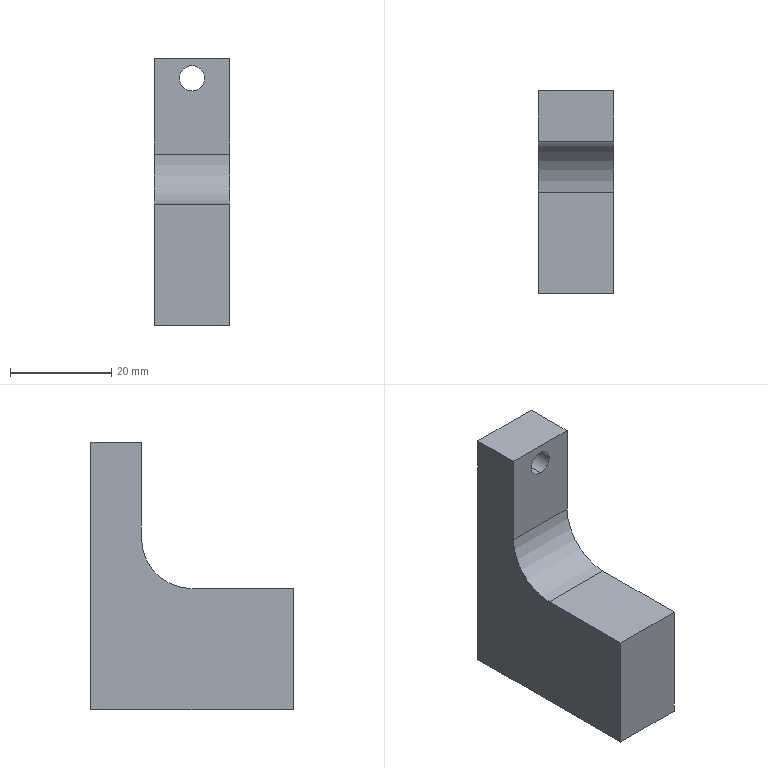Part | STEP file | 11-FG-E02111 | 1 solid | 27 faces | box 15 x 40 x 53 mm | volume 17580 mm3 | cylinder 11 | cone 8 | plane 8 | commonest cylinder face diameters 5 x10 20 x1
STEP:
#1=CARTESIAN_POINT('',(-7.5,40.,51.5));
#2=VERTEX_POINT('',#1);
#3=CARTESIAN_POINT('',(-7.5,40.,46.5));
#4=VERTEX_POINT('',#3);
#5=CARTESIAN_POINT('',(-7.5,40.,49.));
#6=DIRECTION('',(0.,-1.,0.));
#7=DIRECTION('',(0.,0.,-1.));
#8=AXIS2_PLACEMENT_3D('',#5,#6,#7);
#9=CIRCLE('',#8,2.5);
#10=EDGE_CURVE('',#2,#4,#9,.T.);
#11=ORIENTED_EDGE('',*,*,#10,.F.);
#12=CARTESIAN_POINT('',(-7.5,30.,51.5));
#13=VERTEX_POINT('',#12);
#14=CARTESIAN_POINT('',(-7.5,30.,51.5));
#15=DIRECTION('',(0.,-1.,0.));
#16=VECTOR('',#15,1000.);
#17=LINE('',#14,#16);
#18=EDGE_CURVE('',#2,#13,#17,.T.);
#19=ORIENTED_EDGE('',*,*,#18,.T.);
#20=CARTESIAN_POINT('',(-7.5,30.,46.5));
#21=VERTEX_POINT('',#20);
#22=CARTESIAN_POINT('',(-7.5,30.,49.));
#23=DIRECTION('',(0.,-1.,0.));
#24=DIRECTION('',(0.,0.,-1.));
#25=AXIS2_PLACEMENT_3D('',#22,#23,#24);
#26=CIRCLE('',#25,2.5);
#27=EDGE_CURVE('',#13,#21,#26,.T.);
#28=ORIENTED_EDGE('',*,*,#27,.T.);
#29=CARTESIAN_POINT('',(-7.5,30.,46.5));
#30=DIRECTION('',(0.,-1.,0.));
#31=VECTOR('',#30,1000.);
#32=LINE('',#29,#31);
#33=EDGE_CURVE('',#4,#21,#32,.T.);
#34=ORIENTED_EDGE('',*,*,#33,.F.);
#35=EDGE_LOOP('',(#11,#19,#28,#34));
#36=FACE_OUTER_BOUND('',#35,.T.);
#37=CARTESIAN_POINT('',(-7.5,30.,49.));
#38=DIRECTION('',(0.,-1.,0.));
#39=DIRECTION('',(0.,0.,-1.));
#40=AXIS2_PLACEMENT_3D('',#37,#38,#39);
#41=CYLINDRICAL_SURFACE('',#40,2.5);
#42=ADVANCED_FACE('',(#36),#41,.F.);
#43=CARTESIAN_POINT('',(-5.,26.,15.));
#44=VERTEX_POINT('',#43);
#45=CARTESIAN_POINT('',(-10.,26.,15.));
#46=VERTEX_POINT('',#45);
#47=CARTESIAN_POINT('',(-7.5,26.,15.));
#48=DIRECTION('',(0.,0.,-1.));
#49=DIRECTION('',(-1.,0.,0.));
#50=AXIS2_PLACEMENT_3D('',#47,#48,#49);
#51=CIRCLE('',#50,2.5);
#52=EDGE_CURVE('',#44,#46,#51,.T.);
#53=ORIENTED_EDGE('',*,*,#52,.F.);
#54=CARTESIAN_POINT('',(-5.,26.,0.));
#55=VERTEX_POINT('',#54);
#56=CARTESIAN_POINT('',(-5.,26.,0.));
#57=DIRECTION('',(0.,0.,-1.));
#58=VECTOR('',#57,1000.);
#59=LINE('',#56,#58);
#60=EDGE_CURVE('',#44,#55,#59,.T.);
#61=ORIENTED_EDGE('',*,*,#60,.T.);
#62=CARTESIAN_POINT('',(-10.,26.,0.));
#63=VERTEX_POINT('',#62);
#64=CARTESIAN_POINT('',(-7.5,26.,0.));
#65=DIRECTION('',(0.,0.,-1.));
#66=DIRECTION('',(-1.,0.,0.));
#67=AXIS2_PLACEMENT_3D('',#64,#65,#66);
#68=CIRCLE('',#67,2.5);
#69=EDGE_CURVE('',#55,#63,#68,.T.);
#70=ORIENTED_EDGE('',*,*,#69,.T.);
#71=CARTESIAN_POINT('',(-10.,26.,0.));
#72=DIRECTION('',(0.,0.,-1.));
#73=VECTOR('',#72,1000.);
#74=LINE('',#71,#73);
#75=EDGE_CURVE('',#46,#63,#74,.T.);
#76=ORIENTED_EDGE('',*,*,#75,.F.);
#77=EDGE_LOOP('',(#53,#61,#70,#76));
#78=FACE_OUTER_BOUND('',#77,.T.);
#79=CARTESIAN_POINT('',(-7.5,26.,0.));
#80=DIRECTION('',(0.,0.,-1.));
#81=DIRECTION('',(-1.,0.,0.));
#82=AXIS2_PLACEMENT_3D('',#79,#80,#81);
#83=CYLINDRICAL_SURFACE('',#82,2.5);
#84=ADVANCED_FACE('',(#78),#83,.F.);
#85=CARTESIAN_POINT('',(-7.5,26.,16.502));
#86=VERTEX_POINT('',#85);
#87=CARTESIAN_POINT('',(-10.,26.,15.));
#88=DIRECTION('',(-0.8572,0.,-0.515));
#89=VECTOR('',#88,1000.);
#90=LINE('',#87,#89);
#91=EDGE_CURVE('',#86,#46,#90,.T.);
#92=ORIENTED_EDGE('',*,*,#91,.F.);
#93=CARTESIAN_POINT('',(-5.,26.,15.));
#94=DIRECTION('',(0.8572,0.,-0.515));
#95=VECTOR('',#94,1000.);
#96=LINE('',#93,#95);
#97=EDGE_CURVE('',#86,#44,#96,.T.);
#98=ORIENTED_EDGE('',*,*,#97,.T.);
#99=ORIENTED_EDGE('',*,*,#52,.T.);
#100=EDGE_LOOP('',(#92,#98,#99));
#101=FACE_OUTER_BOUND('',#100,.T.);
#102=CARTESIAN_POINT('',(-7.5,26.,15.));
#103=DIRECTION('',(0.,0.,-1.));
#104=DIRECTION('',(-1.,0.,0.));
#105=AXIS2_PLACEMENT_3D('',#102,#103,#104);
#106=CONICAL_SURFACE('',#105,2.5,1.03);
#107=ADVANCED_FACE('',(#101),#106,.F.);
#108=CARTESIAN_POINT('',(-5.,14.,15.));
#109=VERTEX_POINT('',#108);
#110=CARTESIAN_POINT('',(-10.,14.,15.));
#111=VERTEX_POINT('',#110);
#112=CARTESIAN_POINT('',(-7.5,14.,15.));
#113=DIRECTION('',(0.,0.,-1.));
#114=DIRECTION('',(-1.,0.,0.));
#115=AXIS2_PLACEMENT_3D('',#112,#113,#114);
#116=CIRCLE('',#115,2.5);
#117=EDGE_CURVE('',#109,#111,#116,.T.);
#118=ORIENTED_EDGE('',*,*,#117,.F.);
#119=CARTESIAN_POINT('',(-5.,14.,0.));
#120=VERTEX_POINT('',#119);
#121=CARTESIAN_POINT('',(-5.,14.,0.));
#122=DIRECTION('',(0.,0.,-1.));
#123=VECTOR('',#122,1000.);
#124=LINE('',#121,#123);
#125=EDGE_CURVE('',#109,#120,#124,.T.);
#126=ORIENTED_EDGE('',*,*,#125,.T.);
#127=CARTESIAN_POINT('',(-10.,14.,0.));
#128=VERTEX_POINT('',#127);
#129=CARTESIAN_POINT('',(-7.5,14.,0.));
#130=DIRECTION('',(0.,0.,-1.));
#131=DIRECTION('',(-1.,0.,0.));
#132=AXIS2_PLACEMENT_3D('',#129,#130,#131);
#133=CIRCLE('',#132,2.5);
#134=EDGE_CURVE('',#120,#128,#133,.T.);
#135=ORIENTED_EDGE('',*,*,#134,.T.);
#136=CARTESIAN_POINT('',(-10.,14.,0.));
#137=DIRECTION('',(0.,0.,-1.));
#138=VECTOR('',#137,1000.);
#139=LINE('',#136,#138);
#140=EDGE_CURVE('',#111,#128,#139,.T.);
#141=ORIENTED_EDGE('',*,*,#140,.F.);
#142=EDGE_LOOP('',(#118,#126,#135,#141));
#143=FACE_OUTER_BOUND('',#142,.T.);
#144=CARTESIAN_POINT('',(-7.5,14.,0.));
#145=DIRECTION('',(0.,0.,-1.));
#146=DIRECTION('',(-1.,0.,0.));
#147=AXIS2_PLACEMENT_3D('',#144,#145,#146);
#148=CYLINDRICAL_SURFACE('',#147,2.5);
#149=ADVANCED_FACE('',(#143),#148,.F.);
#150=CARTESIAN_POINT('',(-7.5,14.,16.502));
#151=VERTEX_POINT('',#150);
#152=CARTESIAN_POINT('',(-10.,14.,15.));
#153=DIRECTION('',(-0.8572,0.,-0.515));
#154=VECTOR('',#153,1000.);
#155=LINE('',#152,#154);
#156=EDGE_CURVE('',#151,#111,#155,.T.);
#157=ORIENTED_EDGE('',*,*,#156,.F.);
#158=CARTESIAN_POINT('',(-5.,14.,15.));
#159=DIRECTION('',(0.8572,0.,-0.515));
#160=VECTOR('',#159,1000.);
#161=LINE('',#158,#160);
#162=EDGE_CURVE('',#151,#109,#161,.T.);
#163=ORIENTED_EDGE('',*,*,#162,.T.);
#164=ORIENTED_EDGE('',*,*,#117,.T.);
#165=EDGE_LOOP('',(#157,#163,#164));
#166=FACE_OUTER_BOUND('',#165,.T.);
#167=CARTESIAN_POINT('',(-7.5,14.,15.));
#168=DIRECTION('',(0.,0.,-1.));
#169=DIRECTION('',(-1.,0.,0.));
#170=AXIS2_PLACEMENT_3D('',#167,#168,#169);
#171=CONICAL_SURFACE('',#170,2.5,1.03);
#172=ADVANCED_FACE('',(#166),#171,.F.);
#173=CARTESIAN_POINT('',(-5.,35.,17.));
#174=VERTEX_POINT('',#173);
#175=CARTESIAN_POINT('',(-10.,35.,17.));
#176=VERTEX_POINT('',#175);
#177=CARTESIAN_POINT('',(-7.5,35.,17.));
#178=DIRECTION('',(0.,0.,-1.));
#179=DIRECTION('',(-1.,0.,0.));
#180=AXIS2_PLACEMENT_3D('',#177,#178,#179);
#181=CIRCLE('',#180,2.5);
#182=EDGE_CURVE('',#174,#176,#181,.T.);
#183=ORIENTED_EDGE('',*,*,#182,.F.);
#184=CARTESIAN_POINT('',(-5.,35.,0.));
#185=VERTEX_POINT('',#184);
#186=CARTESIAN_POINT('',(-5.,35.,0.));
#187=DIRECTION('',(0.,0.,-1.));
#188=VECTOR('',#187,1000.);
#189=LINE('',#186,#188);
#190=EDGE_CURVE('',#174,#185,#189,.T.);
#191=ORIENTED_EDGE('',*,*,#190,.T.);
#192=CARTESIAN_POINT('',(-10.,35.,0.));
#193=VERTEX_POINT('',#192);
#194=CARTESIAN_POINT('',(-7.5,35.,0.));
#195=DIRECTION('',(0.,0.,-1.));
#196=DIRECTION('',(-1.,0.,0.));
#197=AXIS2_PLACEMENT_3D('',#194,#195,#196);
#198=CIRCLE('',#197,2.5);
#199=EDGE_CURVE('',#185,#193,#198,.T.);
#200=ORIENTED_EDGE('',*,*,#199,.T.);
#201=CARTESIAN_POINT('',(-10.,35.,0.));
#202=DIRECTION('',(0.,0.,-1.));
#203=VECTOR('',#202,1000.);
#204=LINE('',#201,#203);
#205=EDGE_CURVE('',#176,#193,#204,.T.);
#206=ORIENTED_EDGE('',*,*,#205,.F.);
#207=EDGE_LOOP('',(#183,#191,#200,#206));
#208=FACE_OUTER_BOUND('',#207,.T.);
#209=CARTESIAN_POINT('',(-7.5,35.,0.));
#210=DIRECTION('',(0.,0.,-1.));
#211=DIRECTION('',(-1.,0.,0.));
#212=AXIS2_PLACEMENT_3D('',#209,#210,#211);
#213=CYLINDRICAL_SURFACE('',#212,2.5);
#214=ADVANCED_FACE('',(#208),#213,.F.);
#215=CARTESIAN_POINT('',(-7.5,35.,18.502));
#216=VERTEX_POINT('',#215);
#217=CARTESIAN_POINT('',(-10.,35.,17.));
#218=DIRECTION('',(-0.8572,0.,-0.515));
#219=VECTOR('',#218,1000.);
#220=LINE('',#217,#219);
#221=EDGE_CURVE('',#216,#176,#220,.T.);
#222=ORIENTED_EDGE('',*,*,#221,.F.);
#223=CARTESIAN_POINT('',(-5.,35.,17.));
#224=DIRECTION('',(0.8572,0.,-0.515));
#225=VECTOR('',#224,1000.);
#226=LINE('',#223,#225);
#227=EDGE_CURVE('',#216,#174,#226,.T.);
#228=ORIENTED_EDGE('',*,*,#227,.T.);
#229=ORIENTED_EDGE('',*,*,#182,.T.);
#230=EDGE_LOOP('',(#222,#228,#229));
#231=FACE_OUTER_BOUND('',#230,.T.);
#232=CARTESIAN_POINT('',(-7.5,35.,17.));
#233=DIRECTION('',(0.,0.,-1.));
#234=DIRECTION('',(-1.,0.,0.));
#235=AXIS2_PLACEMENT_3D('',#232,#233,#234);
#236=CONICAL_SURFACE('',#235,2.5,1.03);
#237=ADVANCED_FACE('',(#231),#236,.F.);
#238=CARTESIAN_POINT('',(-5.,5.,17.));
#239=VERTEX_POINT('',#238);
#240=CARTESIAN_POINT('',(-10.,5.,17.));
#241=VERTEX_POINT('',#240);
#242=CARTESIAN_POINT('',(-7.5,5.,17.));
#243=DIRECTION('',(0.,0.,-1.));
#244=DIRECTION('',(-1.,0.,0.));
#245=AXIS2_PLACEMENT_3D('',#242,#243,#244);
#246=CIRCLE('',#245,2.5);
#247=EDGE_CURVE('',#239,#241,#246,.T.);
#248=ORIENTED_EDGE('',*,*,#247,.F.);
#249=CARTESIAN_POINT('',(-5.,5.,0.));
#250=VERTEX_POINT('',#249);
#251=CARTESIAN_POINT('',(-5.,5.,0.));
#252=DIRECTION('',(0.,0.,-1.));
#253=VECTOR('',#252,1000.);
#254=LINE('',#251,#253);
#255=EDGE_CURVE('',#239,#250,#254,.T.);
#256=ORIENTED_EDGE('',*,*,#255,.T.);
#257=CARTESIAN_POINT('',(-10.,5.,0.));
#258=VERTEX_POINT('',#257);
#259=CARTESIAN_POINT('',(-7.5,5.,0.));
#260=DIRECTION('',(0.,0.,-1.));
#261=DIRECTION('',(-1.,0.,0.));
#262=AXIS2_PLACEMENT_3D('',#259,#260,#261);
#263=CIRCLE('',#262,2.5);
#264=EDGE_CURVE('',#250,#258,#263,.T.);
#265=ORIENTED_EDGE('',*,*,#264,.T.);
#266=CARTESIAN_POINT('',(-10.,5.,0.));
#267=DIRECTION('',(0.,0.,-1.));
#268=VECTOR('',#267,1000.);
#269=LINE('',#266,#268);
#270=EDGE_CURVE('',#241,#258,#269,.T.);
#271=ORIENTED_EDGE('',*,*,#270,.F.);
#272=EDGE_LOOP('',(#248,#256,#265,#271));
#273=FACE_OUTER_BOUND('',#272,.T.);
#274=CARTESIAN_POINT('',(-7.5,5.,0.));
#275=DIRECTION('',(0.,0.,-1.));
#276=DIRECTION('',(-1.,0.,0.));
#277=AXIS2_PLACEMENT_3D('',#274,#275,#276);
#278=CYLINDRICAL_SURFACE('',#277,2.5);
#279=ADVANCED_FACE('',(#273),#278,.F.);
#280=CARTESIAN_POINT('',(-7.5,5.,18.502));
#281=VERTEX_POINT('',#280);
#282=CARTESIAN_POINT('',(-10.,5.,17.));
#283=DIRECTION('',(-0.8572,0.,-0.515));
#284=VECTOR('',#283,1000.);
#285=LINE('',#282,#284);
#286=EDGE_CURVE('',#281,#241,#285,.T.);
#287=ORIENTED_EDGE('',*,*,#286,.F.);
#288=CARTESIAN_POINT('',(-5.,5.,17.));
#289=DIRECTION('',(0.8572,0.,-0.515));
#290=VECTOR('',#289,1000.);
#291=LINE('',#288,#290);
#292=EDGE_CURVE('',#281,#239,#291,.T.);
#293=ORIENTED_EDGE('',*,*,#292,.T.);
#294=ORIENTED_EDGE('',*,*,#247,.T.);
#295=EDGE_LOOP('',(#287,#293,#294));
#296=FACE_OUTER_BOUND('',#295,.T.);
#297=CARTESIAN_POINT('',(-7.5,5.,17.));
#298=DIRECTION('',(0.,0.,-1.));
#299=DIRECTION('',(-1.,0.,0.));
#300=AXIS2_PLACEMENT_3D('',#297,#298,#299);
#301=CONICAL_SURFACE('',#300,2.5,1.03);
#302=ADVANCED_FACE('',(#296),#301,.F.);
#303=CARTESIAN_POINT('',(0.,30.,53.));
#304=VERTEX_POINT('',#303);
#305=CARTESIAN_POINT('',(0.,40.,53.));
#306=VERTEX_POINT('',#305);
#307=CARTESIAN_POINT('',(0.,0.,53.));
#308=DIRECTION('',(0.,1.,0.));
#309=VECTOR('',#308,1000.);
#310=LINE('',#307,#309);
#311=EDGE_CURVE('',#304,#306,#310,.T.);
#312=ORIENTED_EDGE('',*,*,#311,.F.);
#313=CARTESIAN_POINT('',(0.,30.,34.));
#314=VERTEX_POINT('',#313);
#315=CARTESIAN_POINT('',(0.,30.,53.));
#316=DIRECTION('',(0.,0.,1.));
#317=VECTOR('',#316,1000.);
#318=LINE('',#315,#317);
#319=EDGE_CURVE('',#314,#304,#318,.T.);
#320=ORIENTED_EDGE('',*,*,#319,.F.);
#321=CARTESIAN_POINT('',(0.,20.,24.));
#322=VERTEX_POINT('',#321);
#323=CARTESIAN_POINT('',(0.,20.,34.));
#324=DIRECTION('',(-1.,0.,0.));
#325=DIRECTION('',(0.,0.,1.));
#326=AXIS2_PLACEMENT_3D('',#323,#324,#325);
#327=CIRCLE('',#326,10.);
#328=EDGE_CURVE('',#314,#322,#327,.T.);
#329=ORIENTED_EDGE('',*,*,#328,.T.);
#330=CARTESIAN_POINT('',(0.,0.,24.));
#331=VERTEX_POINT('',#330);
#332=CARTESIAN_POINT('',(0.,0.,24.));
#333=DIRECTION('',(0.,1.,0.));
#334=VECTOR('',#333,1000.);
#335=LINE('',#332,#334);
#336=EDGE_CURVE('',#331,#322,#335,.T.);
#337=ORIENTED_EDGE('',*,*,#336,.F.);
#338=CARTESIAN_POINT('',(0.,0.,0.));
#339=VERTEX_POINT('',#338);
#340=CARTESIAN_POINT('',(0.,0.,53.));
#341=DIRECTION('',(0.,0.,-1.));
#342=VECTOR('',#341,1000.);
#343=LINE('',#340,#342);
#344=EDGE_CURVE('',#331,#339,#343,.T.);
#345=ORIENTED_EDGE('',*,*,#344,.T.);
#346=CARTESIAN_POINT('',(0.,40.,0.));
#347=VERTEX_POINT('',#346);
#348=CARTESIAN_POINT('',(0.,0.,0.));
#349=DIRECTION('',(0.,1.,0.));
#350=VECTOR('',#349,1000.);
#351=LINE('',#348,#350);
#352=EDGE_CURVE('',#339,#347,#351,.T.);
#353=ORIENTED_EDGE('',*,*,#352,.T.);
#354=CARTESIAN_POINT('',(0.,40.,53.));
#355=DIRECTION('',(0.,0.,-1.));
#356=VECTOR('',#355,1000.);
#357=LINE('',#354,#356);
#358=EDGE_CURVE('',#306,#347,#357,.T.);
#359=ORIENTED_EDGE('',*,*,#358,.F.);
#360=EDGE_LOOP('',(#312,#320,#329,#337,#345,#353,#359));
#361=FACE_OUTER_BOUND('',#360,.T.);
#362=CARTESIAN_POINT('',(0.,0.,53.));
#363=DIRECTION('',(-1.,0.,0.));
#364=DIRECTION('',(0.,0.,1.));
#365=AXIS2_PLACEMENT_3D('',#362,#363,#364);
#366=PLANE('',#365);
#367=ADVANCED_FACE('',(#361),#366,.F.);
#368=CARTESIAN_POINT('',(-7.5,40.,49.));
#369=DIRECTION('',(0.,-1.,0.));
#370=DIRECTION('',(0.,0.,-1.));
#371=AXIS2_PLACEMENT_3D('',#368,#369,#370);
#372=CIRCLE('',#371,2.5);
#373=EDGE_CURVE('',#4,#2,#372,.T.);
#374=ORIENTED_EDGE('',*,*,#373,.T.);
#375=ORIENTED_EDGE('',*,*,#10,.T.);
#376=EDGE_LOOP('',(#374,#375));
#377=FACE_BOUND('',#376,.T.);
#378=CARTESIAN_POINT('',(-15.,40.,0.));
#379=VERTEX_POINT('',#378);
#380=CARTESIAN_POINT('',(0.,40.,0.));
#381=DIRECTION('',(-1.,0.,0.));
#382=VECTOR('',#381,1000.);
#383=LINE('',#380,#382);
#384=EDGE_CURVE('',#347,#379,#383,.T.);
#385=ORIENTED_EDGE('',*,*,#384,.T.);
#386=CARTESIAN_POINT('',(-15.,40.,53.));
#387=VERTEX_POINT('',#386);
#388=CARTESIAN_POINT('',(-15.,40.,53.));
#389=DIRECTION('',(0.,0.,-1.));
#390=VECTOR('',#389,1000.);
#391=LINE('',#388,#390);
#392=EDGE_CURVE('',#387,#379,#391,.T.);
#393=ORIENTED_EDGE('',*,*,#392,.F.);
#394=CARTESIAN_POINT('',(0.,40.,53.));
#395=DIRECTION('',(-1.,0.,0.));
#396=VECTOR('',#395,1000.);
#397=LINE('',#394,#396);
#398=EDGE_CURVE('',#306,#387,#397,.T.);
#399=ORIENTED_EDGE('',*,*,#398,.F.);
#400=ORIENTED_EDGE('',*,*,#358,.T.);
#401=EDGE_LOOP('',(#385,#393,#399,#400));
#402=FACE_OUTER_BOUND('',#401,.T.);
#403=CARTESIAN_POINT('',(0.,40.,53.));
#404=DIRECTION('',(0.,-1.,0.));
#405=DIRECTION('',(0.,0.,-1.));
#406=AXIS2_PLACEMENT_3D('',#403,#404,#405);
#407=PLANE('',#406);
#408=ADVANCED_FACE('',(#377,#402),#407,.F.);
#409=CARTESIAN_POINT('',(-15.,0.,24.));
#410=VERTEX_POINT('',#409);
#411=CARTESIAN_POINT('',(-15.,20.,24.));
#412=VERTEX_POINT('',#411);
#413=CARTESIAN_POINT('',(-15.,0.,24.));
#414=DIRECTION('',(0.,1.,0.));
#415=VECTOR('',#414,1000.);
#416=LINE('',#413,#415);
#417=EDGE_CURVE('',#410,#412,#416,.T.);
#418=ORIENTED_EDGE('',*,*,#417,.T.);
#419=CARTESIAN_POINT('',(-15.,30.,34.));
#420=VERTEX_POINT('',#419);
#421=CARTESIAN_POINT('',(-15.,20.,34.));
#422=DIRECTION('',(1.,0.,0.));
#423=DIRECTION('',(0.,0.,-1.));
#424=AXIS2_PLACEMENT_3D('',#421,#422,#423);
#425=CIRCLE('',#424,10.);
#426=EDGE_CURVE('',#412,#420,#425,.T.);
#427=ORIENTED_EDGE('',*,*,#426,.T.);
#428=CARTESIAN_POINT('',(-15.,30.,53.));
#429=VERTEX_POINT('',#428);
#430=CARTESIAN_POINT('',(-15.,30.,53.));
#431=DIRECTION('',(0.,0.,1.));
#432=VECTOR('',#431,1000.);
#433=LINE('',#430,#432);
#434=EDGE_CURVE('',#420,#429,#433,.T.);
#435=ORIENTED_EDGE('',*,*,#434,.T.);
#436=CARTESIAN_POINT('',(-15.,0.,53.));
#437=DIRECTION('',(0.,-1.,0.));
#438=VECTOR('',#437,1000.);
#439=LINE('',#436,#438);
#440=EDGE_CURVE('',#387,#429,#439,.T.);
#441=ORIENTED_EDGE('',*,*,#440,.F.);
#442=ORIENTED_EDGE('',*,*,#392,.T.);
#443=CARTESIAN_POINT('',(-15.,0.,0.));
#444=VERTEX_POINT('',#443);
#445=CARTESIAN_POINT('',(-15.,0.,0.));
#446=DIRECTION('',(0.,-1.,0.));
#447=VECTOR('',#446,1000.);
#448=LINE('',#445,#447);
#449=EDGE_CURVE('',#379,#444,#448,.T.);
#450=ORIENTED_EDGE('',*,*,#449,.T.);
#451=CARTESIAN_POINT('',(-15.,0.,53.));
#452=DIRECTION('',(0.,0.,-1.));
#453=VECTOR('',#452,1000.);
#454=LINE('',#451,#453);
#455=EDGE_CURVE('',#410,#444,#454,.T.);
#456=ORIENTED_EDGE('',*,*,#455,.F.);
#457=EDGE_LOOP('',(#418,#427,#435,#441,#442,#450,#456));
#458=FACE_OUTER_BOUND('',#457,.T.);
#459=CARTESIAN_POINT('',(-15.,0.,53.));
#460=DIRECTION('',(1.,0.,0.));
#461=DIRECTION('',(0.,0.,-1.));
#462=AXIS2_PLACEMENT_3D('',#459,#460,#461);
#463=PLANE('',#462);
#464=ADVANCED_FACE('',(#458),#463,.F.);
#465=ORIENTED_EDGE('',*,*,#344,.F.);
#466=CARTESIAN_POINT('',(-34.,0.,24.));
#467=DIRECTION('',(1.,0.,0.));
#468=VECTOR('',#467,1000.);
#469=LINE('',#466,#468);
#470=EDGE_CURVE('',#410,#331,#469,.T.);
#471=ORIENTED_EDGE('',*,*,#470,.F.);
#472=ORIENTED_EDGE('',*,*,#455,.T.);
#473=CARTESIAN_POINT('',(0.,0.,0.));
#474=DIRECTION('',(1.,0.,0.));
#475=VECTOR('',#474,1000.);
#476=LINE('',#473,#475);
#477=EDGE_CURVE('',#444,#339,#476,.T.);
#478=ORIENTED_EDGE('',*,*,#477,.T.);
#479=EDGE_LOOP('',(#465,#471,#472,#478));
#480=FACE_OUTER_BOUND('',#479,.T.);
#481=CARTESIAN_POINT('',(0.,0.,53.));
#482=DIRECTION('',(0.,1.,0.));
#483=DIRECTION('',(-1.,0.,0.));
#484=AXIS2_PLACEMENT_3D('',#481,#482,#483);
#485=PLANE('',#484);
#486=ADVANCED_FACE('',(#480),#485,.F.);
#487=CARTESIAN_POINT('',(0.,30.,53.));
#488=DIRECTION('',(-1.,0.,0.));
#489=VECTOR('',#488,1000.);
#490=LINE('',#487,#489);
#491=EDGE_CURVE('',#304,#429,#490,.T.);
#492=ORIENTED_EDGE('',*,*,#491,.F.);
#493=ORIENTED_EDGE('',*,*,#311,.T.);
#494=ORIENTED_EDGE('',*,*,#398,.T.);
#495=ORIENTED_EDGE('',*,*,#440,.T.);
#496=EDGE_LOOP('',(#492,#493,#494,#495));
#497=FACE_OUTER_BOUND('',#496,.T.);
#498=CARTESIAN_POINT('',(0.,40.,53.));
#499=DIRECTION('',(0.,0.,1.));
#500=DIRECTION('',(1.,0.,0.));
#501=AXIS2_PLACEMENT_3D('',#498,#499,#500);
#502=PLANE('',#501);
#503=ADVANCED_FACE('',(#497),#502,.T.);
#504=CARTESIAN_POINT('',(-7.5,26.,0.));
#505=DIRECTION('',(0.,0.,-1.));
#506=DIRECTION('',(-1.,0.,0.));
#507=AXIS2_PLACEMENT_3D('',#504,#505,#506);
#508=CIRCLE('',#507,2.5);
#509=EDGE_CURVE('',#63,#55,#508,.T.);
#510=ORIENTED_EDGE('',*,*,#509,.F.);
#511=ORIENTED_EDGE('',*,*,#69,.F.);
#512=EDGE_LOOP('',(#510,#511));
#513=FACE_BOUND('',#512,.T.);
#514=CARTESIAN_POINT('',(-7.5,14.,0.));
#515=DIRECTION('',(0.,0.,-1.));
#516=DIRECTION('',(-1.,0.,0.));
#517=AXIS2_PLACEMENT_3D('',#514,#515,#516);
#518=CIRCLE('',#517,2.5);
#519=EDGE_CURVE('',#128,#120,#518,.T.);
#520=ORIENTED_EDGE('',*,*,#519,.F.);
#521=ORIENTED_EDGE('',*,*,#134,.F.);
#522=EDGE_LOOP('',(#520,#521));
#523=FACE_BOUND('',#522,.T.);
#524=CARTESIAN_POINT('',(-7.5,35.,0.));
#525=DIRECTION('',(0.,0.,-1.));
#526=DIRECTION('',(-1.,0.,0.));
#527=AXIS2_PLACEMENT_3D('',#524,#525,#526);
#528=CIRCLE('',#527,2.5);
#529=EDGE_CURVE('',#193,#185,#528,.T.);
#530=ORIENTED_EDGE('',*,*,#529,.F.);
#531=ORIENTED_EDGE('',*,*,#199,.F.);
#532=EDGE_LOOP('',(#530,#531));
#533=FACE_BOUND('',#532,.T.);
#534=CARTESIAN_POINT('',(-7.5,5.,0.));
#535=DIRECTION('',(0.,0.,-1.));
#536=DIRECTION('',(-1.,0.,0.));
#537=AXIS2_PLACEMENT_3D('',#534,#535,#536);
#538=CIRCLE('',#537,2.5);
#539=EDGE_CURVE('',#258,#250,#538,.T.);
#540=ORIENTED_EDGE('',*,*,#539,.F.);
#541=ORIENTED_EDGE('',*,*,#264,.F.);
#542=EDGE_LOOP('',(#540,#541));
#543=FACE_BOUND('',#542,.T.);
#544=ORIENTED_EDGE('',*,*,#352,.F.);
#545=ORIENTED_EDGE('',*,*,#477,.F.);
#546=ORIENTED_EDGE('',*,*,#449,.F.);
#547=ORIENTED_EDGE('',*,*,#384,.F.);
#548=EDGE_LOOP('',(#544,#545,#546,#547));
#549=FACE_OUTER_BOUND('',#548,.T.);
#550=CARTESIAN_POINT('',(0.,40.,0.));
#551=DIRECTION('',(0.,0.,1.));
#552=DIRECTION('',(1.,0.,0.));
#553=AXIS2_PLACEMENT_3D('',#550,#551,#552);
#554=PLANE('',#553);
#555=ADVANCED_FACE('',(#513,#523,#533,#543,#549),#554,.F.);
#556=ORIENTED_EDGE('',*,*,#336,.T.);
#557=CARTESIAN_POINT('',(-15.,20.,24.));
#558=DIRECTION('',(-1.,0.,0.));
#559=VECTOR('',#558,1000.);
#560=LINE('',#557,#559);
#561=EDGE_CURVE('',#322,#412,#560,.T.);
#562=ORIENTED_EDGE('',*,*,#561,.T.);
#563=ORIENTED_EDGE('',*,*,#417,.F.);
#564=ORIENTED_EDGE('',*,*,#470,.T.);
#565=EDGE_LOOP('',(#556,#562,#563,#564));
#566=FACE_OUTER_BOUND('',#565,.T.);
#567=CARTESIAN_POINT('',(-34.,0.,24.));
#568=DIRECTION('',(0.,0.,-1.));
#569=DIRECTION('',(-1.,0.,0.));
#570=AXIS2_PLACEMENT_3D('',#567,#568,#569);
#571=PLANE('',#570);
#572=ADVANCED_FACE('',(#566),#571,.F.);
#573=CARTESIAN_POINT('',(-7.5,30.,49.));
#574=DIRECTION('',(0.,-1.,0.));
#575=DIRECTION('',(0.,0.,-1.));
#576=AXIS2_PLACEMENT_3D('',#573,#574,#575);
#577=CIRCLE('',#576,2.5);
#578=EDGE_CURVE('',#21,#13,#577,.T.);
#579=ORIENTED_EDGE('',*,*,#578,.F.);
#580=ORIENTED_EDGE('',*,*,#27,.F.);
#581=EDGE_LOOP('',(#579,#580));
#582=FACE_BOUND('',#581,.T.);
#583=ORIENTED_EDGE('',*,*,#434,.F.);
#584=CARTESIAN_POINT('',(0.,30.,34.));
#585=DIRECTION('',(1.,0.,0.));
#586=VECTOR('',#585,1000.);
#587=LINE('',#584,#586);
#588=EDGE_CURVE('',#420,#314,#587,.T.);
#589=ORIENTED_EDGE('',*,*,#588,.T.);
#590=ORIENTED_EDGE('',*,*,#319,.T.);
#591=ORIENTED_EDGE('',*,*,#491,.T.);
#592=EDGE_LOOP('',(#583,#589,#590,#591));
#593=FACE_OUTER_BOUND('',#592,.T.);
#594=CARTESIAN_POINT('',(-34.,30.,53.));
#595=DIRECTION('',(0.,1.,0.));
#596=DIRECTION('',(0.,0.,1.));
#597=AXIS2_PLACEMENT_3D('',#594,#595,#596);
#598=PLANE('',#597);
#599=ADVANCED_FACE('',(#582,#593),#598,.F.);
#600=ORIENTED_EDGE('',*,*,#426,.F.);
#601=ORIENTED_EDGE('',*,*,#561,.F.);
#602=ORIENTED_EDGE('',*,*,#328,.F.);
#603=ORIENTED_EDGE('',*,*,#588,.F.);
#604=EDGE_LOOP('',(#600,#601,#602,#603));
#605=FACE_OUTER_BOUND('',#604,.T.);
#606=CARTESIAN_POINT('',(-34.,20.,34.));
#607=DIRECTION('',(-1.,0.,0.));
#608=DIRECTION('',(0.,0.,1.));
#609=AXIS2_PLACEMENT_3D('',#606,#607,#608);
#610=CYLINDRICAL_SURFACE('',#609,10.);
#611=ADVANCED_FACE('',(#605),#610,.F.);
#612=ORIENTED_EDGE('',*,*,#292,.F.);
#613=ORIENTED_EDGE('',*,*,#286,.T.);
#614=CARTESIAN_POINT('',(-7.5,5.,17.));
#615=DIRECTION('',(0.,0.,-1.));
#616=DIRECTION('',(-1.,0.,0.));
#617=AXIS2_PLACEMENT_3D('',#614,#615,#616);
#618=CIRCLE('',#617,2.5);
#619=EDGE_CURVE('',#241,#239,#618,.T.);
#620=ORIENTED_EDGE('',*,*,#619,.T.);
#621=EDGE_LOOP('',(#612,#613,#620));
#622=FACE_OUTER_BOUND('',#621,.T.);
#623=CARTESIAN_POINT('',(-7.5,5.,17.));
#624=DIRECTION('',(0.,0.,-1.));
#625=DIRECTION('',(-1.,0.,0.));
#626=AXIS2_PLACEMENT_3D('',#623,#624,#625);
#627=CONICAL_SURFACE('',#626,2.5,1.03);
#628=ADVANCED_FACE('',(#622),#627,.F.);
#629=ORIENTED_EDGE('',*,*,#255,.F.);
#630=ORIENTED_EDGE('',*,*,#619,.F.);
#631=ORIENTED_EDGE('',*,*,#270,.T.);
#632=ORIENTED_EDGE('',*,*,#539,.T.);
#633=EDGE_LOOP('',(#629,#630,#631,#632));
#634=FACE_OUTER_BOUND('',#633,.T.);
#635=CARTESIAN_POINT('',(-7.5,5.,0.));
#636=DIRECTION('',(0.,0.,-1.));
#637=DIRECTION('',(-1.,0.,0.));
#638=AXIS2_PLACEMENT_3D('',#635,#636,#637);
#639=CYLINDRICAL_SURFACE('',#638,2.5);
#640=ADVANCED_FACE('',(#634),#639,.F.);
#641=ORIENTED_EDGE('',*,*,#227,.F.);
#642=ORIENTED_EDGE('',*,*,#221,.T.);
#643=CARTESIAN_POINT('',(-7.5,35.,17.));
#644=DIRECTION('',(0.,0.,-1.));
#645=DIRECTION('',(-1.,0.,0.));
#646=AXIS2_PLACEMENT_3D('',#643,#644,#645);
#647=CIRCLE('',#646,2.5);
#648=EDGE_CURVE('',#176,#174,#647,.T.);
#649=ORIENTED_EDGE('',*,*,#648,.T.);
#650=EDGE_LOOP('',(#641,#642,#649));
#651=FACE_OUTER_BOUND('',#650,.T.);
#652=CARTESIAN_POINT('',(-7.5,35.,17.));
#653=DIRECTION('',(0.,0.,-1.));
#654=DIRECTION('',(-1.,0.,0.));
#655=AXIS2_PLACEMENT_3D('',#652,#653,#654);
#656=CONICAL_SURFACE('',#655,2.5,1.03);
#657=ADVANCED_FACE('',(#651),#656,.F.);
#658=ORIENTED_EDGE('',*,*,#190,.F.);
#659=ORIENTED_EDGE('',*,*,#648,.F.);
#660=ORIENTED_EDGE('',*,*,#205,.T.);
#661=ORIENTED_EDGE('',*,*,#529,.T.);
#662=EDGE_LOOP('',(#658,#659,#660,#661));
#663=FACE_OUTER_BOUND('',#662,.T.);
#664=CARTESIAN_POINT('',(-7.5,35.,0.));
#665=DIRECTION('',(0.,0.,-1.));
#666=DIRECTION('',(-1.,0.,0.));
#667=AXIS2_PLACEMENT_3D('',#664,#665,#666);
#668=CYLINDRICAL_SURFACE('',#667,2.5);
#669=ADVANCED_FACE('',(#663),#668,.F.);
#670=ORIENTED_EDGE('',*,*,#162,.F.);
#671=ORIENTED_EDGE('',*,*,#156,.T.);
#672=CARTESIAN_POINT('',(-7.5,14.,15.));
#673=DIRECTION('',(0.,0.,-1.));
#674=DIRECTION('',(-1.,0.,0.));
#675=AXIS2_PLACEMENT_3D('',#672,#673,#674);
#676=CIRCLE('',#675,2.5);
#677=EDGE_CURVE('',#111,#109,#676,.T.);
#678=ORIENTED_EDGE('',*,*,#677,.T.);
#679=EDGE_LOOP('',(#670,#671,#678));
#680=FACE_OUTER_BOUND('',#679,.T.);
#681=CARTESIAN_POINT('',(-7.5,14.,15.));
#682=DIRECTION('',(0.,0.,-1.));
#683=DIRECTION('',(-1.,0.,0.));
#684=AXIS2_PLACEMENT_3D('',#681,#682,#683);
#685=CONICAL_SURFACE('',#684,2.5,1.03);
#686=ADVANCED_FACE('',(#680),#685,.F.);
#687=ORIENTED_EDGE('',*,*,#125,.F.);
#688=ORIENTED_EDGE('',*,*,#677,.F.);
#689=ORIENTED_EDGE('',*,*,#140,.T.);
#690=ORIENTED_EDGE('',*,*,#519,.T.);
#691=EDGE_LOOP('',(#687,#688,#689,#690));
#692=FACE_OUTER_BOUND('',#691,.T.);
#693=CARTESIAN_POINT('',(-7.5,14.,0.));
#694=DIRECTION('',(0.,0.,-1.));
#695=DIRECTION('',(-1.,0.,0.));
#696=AXIS2_PLACEMENT_3D('',#693,#694,#695);
#697=CYLINDRICAL_SURFACE('',#696,2.5);
#698=ADVANCED_FACE('',(#692),#697,.F.);
#699=ORIENTED_EDGE('',*,*,#97,.F.);
#700=ORIENTED_EDGE('',*,*,#91,.T.);
#701=CARTESIAN_POINT('',(-7.5,26.,15.));
#702=DIRECTION('',(0.,0.,-1.));
#703=DIRECTION('',(-1.,0.,0.));
#704=AXIS2_PLACEMENT_3D('',#701,#702,#703);
#705=CIRCLE('',#704,2.5);
#706=EDGE_CURVE('',#46,#44,#705,.T.);
#707=ORIENTED_EDGE('',*,*,#706,.T.);
#708=EDGE_LOOP('',(#699,#700,#707));
#709=FACE_OUTER_BOUND('',#708,.T.);
#710=CARTESIAN_POINT('',(-7.5,26.,15.));
#711=DIRECTION('',(0.,0.,-1.));
#712=DIRECTION('',(-1.,0.,0.));
#713=AXIS2_PLACEMENT_3D('',#710,#711,#712);
#714=CONICAL_SURFACE('',#713,2.5,1.03);
#715=ADVANCED_FACE('',(#709),#714,.F.);
#716=ORIENTED_EDGE('',*,*,#60,.F.);
#717=ORIENTED_EDGE('',*,*,#706,.F.);
#718=ORIENTED_EDGE('',*,*,#75,.T.);
#719=ORIENTED_EDGE('',*,*,#509,.T.);
#720=EDGE_LOOP('',(#716,#717,#718,#719));
#721=FACE_OUTER_BOUND('',#720,.T.);
#722=CARTESIAN_POINT('',(-7.5,26.,0.));
#723=DIRECTION('',(0.,0.,-1.));
#724=DIRECTION('',(-1.,0.,0.));
#725=AXIS2_PLACEMENT_3D('',#722,#723,#724);
#726=CYLINDRICAL_SURFACE('',#725,2.5);
#727=ADVANCED_FACE('',(#721),#726,.F.);
#728=ORIENTED_EDGE('',*,*,#18,.F.);
#729=ORIENTED_EDGE('',*,*,#373,.F.);
#730=ORIENTED_EDGE('',*,*,#33,.T.);
#731=ORIENTED_EDGE('',*,*,#578,.T.);
#732=EDGE_LOOP('',(#728,#729,#730,#731));
#733=FACE_OUTER_BOUND('',#732,.T.);
#734=CARTESIAN_POINT('',(-7.5,30.,49.));
#735=DIRECTION('',(0.,-1.,0.));
#736=DIRECTION('',(0.,0.,-1.));
#737=AXIS2_PLACEMENT_3D('',#734,#735,#736);
#738=CYLINDRICAL_SURFACE('',#737,2.5);
#739=ADVANCED_FACE('',(#733),#738,.F.);
#740=CLOSED_SHELL('',(#42,#84,#107,#149,#172,#214,#237,#279,#302,#367,#408,#464,#486,#503,#555,#572,#599,#611,#628,#640,#657,#669,#686,#698,#715,#727,#739));
#741=MANIFOLD_SOLID_BREP('',#740);
#742=CARTESIAN_POINT('',(0.,0.,0.));
#743=DIRECTION('',(0.,0.,1.));
#744=DIRECTION('',(1.,0.,0.));
#745=AXIS2_PLACEMENT_3D('',#742,#743,#744);
#746=(LENGTH_UNIT()NAMED_UNIT(*)SI_UNIT(.MILLI.,.METRE.));
#747=UNCERTAINTY_MEASURE_WITH_UNIT(LENGTH_MEASURE(0.00001),#746,'','');
#748=(NAMED_UNIT(*)PLANE_ANGLE_UNIT()SI_UNIT($,.RADIAN.));
#749=(NAMED_UNIT(*)SI_UNIT($,.STERADIAN.)SOLID_ANGLE_UNIT());
#750=(GEOMETRIC_REPRESENTATION_CONTEXT(3)GLOBAL_UNCERTAINTY_ASSIGNED_CONTEXT((#747))GLOBAL_UNIT_ASSIGNED_CONTEXT((#746,#748,#749))REPRESENTATION_CONTEXT('',''));
#751=ADVANCED_BREP_SHAPE_REPRESENTATION('',(#741,#745),#750);